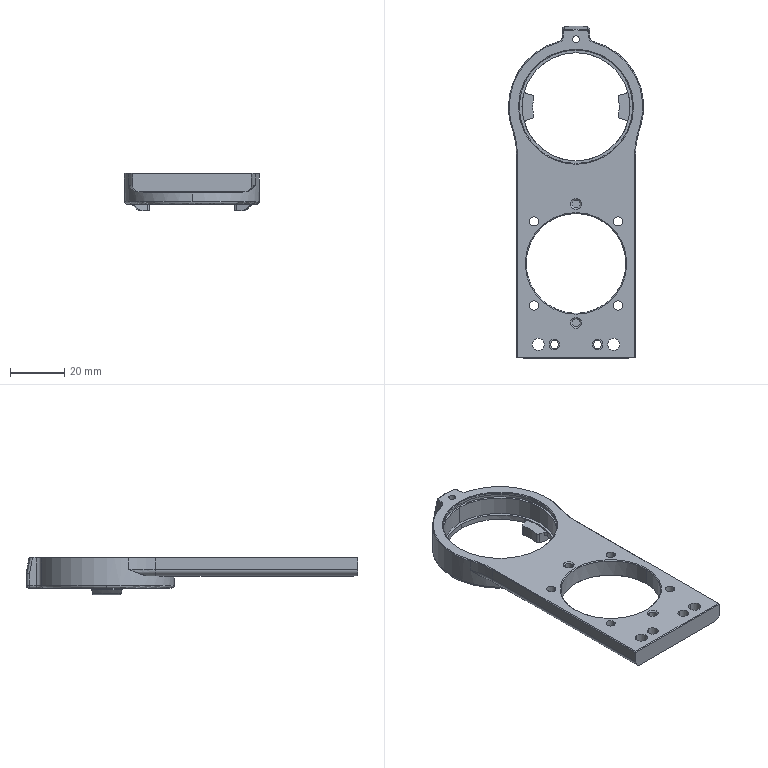NC program | NX | posted with a generic post | part box 50 x 122.9 x 14 mm
Lines 2831 to 4462 of 4462:
(ZLEVEL_PROFILE_COPY , TOOL : D10JING)
N5642 T14 M6
N5644 G54
N5646 G17 G0 G90 X-66.45 Y1.257 S9500 M3
N5648 G43 Z30. H14
N5650 Z-12.5
N5652 G94 G1 Y22.549 Z-13.616 F1000.
N5654 X-66.122 Y23.864 Z-13.687
N5656 X-65.454 Y25.045 Z-13.758
N5658 X-64.495 Y26.004 Z-13.829
N5660 X-63.314 Y26.672 Z-13.9
N5662 X-61.999 Y27. Z-13.971
N5664 X-61.45 Z-14.
N5666 X13.634 F1500.
N5668 G3 X21.777 Y28.364 R25.
N5670 G2 X59.834 Y10. R30.
N5672 G1 X60.172
N5674 G2 X66.114 Y4.83 R6.
N5676 X66.114 Y-4.83 R34.9
N5678 X60.172 Y-10. R6.
N5680 G1 X59.951
N5682 X59.835 Y-9.998
N5684 G2 X21.777 Y-28.364 R30.
N5686 G3 X13.634 Y-27. R25.
N5688 G1 X-61.45
N5690 G2 X-66.45 Y-22. R5.
N5692 G1 Y22.
N5694 G2 X-61.45 Y27. R5.
N5696 G1 Z-12.5
N5698 G0 Z30.
(HOLE_MILLING_COPY_COPY , TOOL : D10JING)
N5700 X31.55 Y0.
N5702 Z0.5
N5704 G41 G1 X27.575 Y-11.323 F1000. D14
N5706 G3 X31.55 Y-16.005 R4.028
N5708 X31.55 Y-16.005 Z-0.5 I0. J16.005 F2000.
N5710 X31.55 Y-16.005 Z-1.5 I0. J16.005
N5712 X31.55 Y-16.005 Z-2.5 I0. J16.005
N5714 X31.55 Y-16.005 Z-3.5 I0. J16.005
N5716 X31.55 Y-16.005 Z-4.5 I0. J16.005
N5718 X31.55 Y-16.005 Z-5.5 I0. J16.005
N5720 X31.55 Y-16.005 Z-6.5 I0. J16.005
N5722 X31.55 Y-16.005 Z-7.5 I0. J16.005
N5724 X31.55 Y-16.005 Z-8.5 I0. J16.005
N5726 X31.55 Y-16.005 Z-9.5 I0. J16.005
N5728 X34.054 Y-15.808 Z-9.525 R16.005
N5730 X47.358 Y2.504 R16.005
N5732 X34.054 Y-15.808 R-16.005
N5734 X37.247 Y-10.561 R4.028
N5736 G40
N5738 G1 X31.55 Y0.
N5740 G0 Z30.
(HOLE_MILLING_COPY_COPY_COPY , TOOL : D10JING)
N5742 Z0.5
N5744 G1 X28.854 Y-12.722 F1000.
N5746 G3 X31.55 Y-16.05 R2.756
N5748 X31.55 Y-16.05 Z-0.5 I0. J16.05 F2000.
N5750 X31.55 Y16.05 Z-1. I0. J16.05
N5752 X15.5 Y0. R16.05
N5754 X31.55 Y16.05 R-16.05
N5756 X28.854 Y12.722 R2.756
N5758 G1 X31.55 Y0.
N5760 G0 Z30.
N5762 M5
(SPOT_DRILLING , TOOL : D6A45)
N5764 T01 M6
N5766 G54
N5768 G17 G0 G90 X-42.006 Y15.556 S9500 M3
N5770 G43 Z30. H1
N5772 G94 G82 G98 Z-1. F250. P200 R3.
N5774 X-56.45 Y14.
N5776 Y8.
N5778 X-48.45 Y0.
N5780 X-56.45 Y-8.
N5782 Y-14.
N5784 X-42.006 Y-15.556
N5786 X-26.45 Y0.
N5788 X-10.894 Y15.556
N5790 X-4.45 Y0.
N5792 X-10.894 Y-15.556
N5794 X31.55 Y0.
N5796 X56.55
N5798 G80
N5800 G0 X56.55 Y0. Z30.
N5802 M5
(DRILLING , TOOL : 4.5ZT)
N5804 T08 M6
N5806 G54
N5808 G17 G0 G90 X-56.45 Y14. S2500 M3
N5810 G43 Z30. H8
N5812 G94 G83 G98 Z-6.452 F200. Q2. R3.
N5814 Y-14.
N5816 G80
N5818 G0 X-56.45 Y-14. Z30.
N5820 M5
(DRILLING_COPY , TOOL : 3.0ZT)
N5822 T16 M6
N5824 G54
N5826 G17 G0 G90 X-56.45 Y8. S2500 M3
N5828 G43 Z30. H16
N5830 G94 G83 G98 Z-9.401 F200. Q2. R3.
N5832 Y-8.
N5834 G80
N5836 G0 X-56.45 Y-8. Z30.
N5838 M5
(DRILLING_COPY_COPY , TOOL : 3.4ZT)
N5840 T07 M6
N5842 G54
N5844 G17 G0 G90 X-42.006 Y15.556 S2500 M3
N5846 G43 Z30. H7
N5848 G94 G83 G98 Z-9.521 F200. Q2. R3.
N5850 Y-15.556
N5852 X-10.894
N5854 Y15.556
N5856 G80
N5858 G0 X-10.894 Y15.556 Z30.
N5860 M5
(DRILLING_COPY_COPY_COPY , TOOL : 2.5ZT)
N5862 T02 M6
N5864 G54
N5866 G17 G0 G90 X56.55 Y0. S2500 M3
N5868 G43 Z30. H2
N5870 G94 G83 G98 Z-13.751 F100. Q2. R3.
N5872 G80
N5874 G0 X56.55 Y0. Z30.
N5876 M5
(HOLE_MILLING_1 , TOOL : D2)
N5878 T17 M6
N5880 G54
N5882 G17 G0 G90 X-56.45 Y8. S9500 M3
N5884 G43 Z30. H17
N5886 Z0.5
N5888 G94 G3 X-56.95 Y7.5 R0.5 F1050.
N5890 X-56.45 Y7. R0.5
N5892 X-56.45 Y7. Z0.35 I0. J1.
N5894 X-56.45 Y7. Z0.2 I0. J1.
N5896 X-56.45 Y7. Z0.05 I0. J1.
N5898 X-56.45 Y7. Z-0.1 I0. J1.
N5900 X-56.45 Y7. Z-0.25 I0. J1.
N5902 X-56.45 Y7. Z-0.4 I0. J1.
N5904 X-56.45 Y7. Z-0.55 I0. J1.
N5906 X-56.45 Y7. Z-0.7 I0. J1.
N5908 X-56.45 Y7. Z-0.85 I0. J1.
N5910 X-56.45 Y7. Z-1. I0. J1.
N5912 X-56.45 Y7. Z-1.15 I0. J1.
N5914 X-56.45 Y7. Z-1.3 I0. J1.
N5916 X-56.45 Y7. Z-1.45 I0. J1.
N5918 X-56.45 Y7. Z-1.6 I0. J1.
N5920 X-56.45 Y7. Z-1.75 I0. J1.
N5922 X-56.45 Y7. Z-1.9 I0. J1.
N5924 X-56.45 Y7. Z-2.05 I0. J1.
N5926 X-56.45 Y7. Z-2.2 I0. J1.
N5928 X-56.45 Y7. Z-2.35 I0. J1.
N5930 X-56.45 Y7. Z-2.5 I0. J1.
N5932 X-56.45 Y7. Z-2.65 I0. J1.
N5934 X-56.45 Y7. Z-2.8 I0. J1.
N5936 X-56.45 Y7. Z-2.95 I0. J1.
N5938 X-56.45 Y7. Z-3.1 I0. J1.
N5940 X-56.45 Y7. Z-3.25 I0. J1.
N5942 X-56.45 Y7. Z-3.4 I0. J1.
N5944 X-56.45 Y7. Z-3.55 I0. J1.
N5946 X-56.45 Y7. Z-3.7 I0. J1.
N5948 X-56.45 Y7. Z-3.85 I0. J1.
N5950 X-56.45 Y7. Z-4. I0. J1.
N5952 X-56.45 Y7. Z-4.15 I0. J1.
N5954 X-56.45 Y7. Z-4.3 I0. J1.
N5956 X-56.45 Y7. Z-4.45 I0. J1.
N5958 X-56.45 Y7. Z-4.6 I0. J1.
N5960 X-56.45 Y7. Z-4.75 I0. J1.
N5962 X-56.45 Y7. Z-4.9 I0. J1.
N5964 X-57.316 Y8.5 Z-5. R-1.
N5966 X-56.95 Y7.134 R1.
N5968 X-57.316 Y8.5 R-1.
N5970 X-57.133 Y7.817 R0.5
N5972 X-56.45 Y8. R0.5
N5974 G0 Z30.
N5976 Y-8.
N5978 Z0.5
N5980 G3 X-56.95 Y-8.5 R0.5
N5982 X-56.45 Y-9. R0.5
N5984 X-56.45 Y-9. Z0.35 I0. J1.
N5986 X-56.45 Y-9. Z0.2 I0. J1.
N5988 X-56.45 Y-9. Z0.05 I0. J1.
N5990 X-56.45 Y-9. Z-0.1 I0. J1.
N5992 X-56.45 Y-9. Z-0.25 I0. J1.
N5994 X-56.45 Y-9. Z-0.4 I0. J1.
N5996 X-56.45 Y-9. Z-0.55 I0. J1.
N5998 X-56.45 Y-9. Z-0.7 I0. J1.
N6000 X-56.45 Y-9. Z-0.85 I0. J1.
N6002 X-56.45 Y-9. Z-1. I0. J1.
N6004 X-56.45 Y-9. Z-1.15 I0. J1.
N6006 X-56.45 Y-9. Z-1.3 I0. J1.
N6008 X-56.45 Y-9. Z-1.45 I0. J1.
N6010 X-56.45 Y-9. Z-1.6 I0. J1.
N6012 X-56.45 Y-9. Z-1.75 I0. J1.
N6014 X-56.45 Y-9. Z-1.9 I0. J1.
N6016 X-56.45 Y-9. Z-2.05 I0. J1.
N6018 X-56.45 Y-9. Z-2.2 I0. J1.
N6020 X-56.45 Y-9. Z-2.35 I0. J1.
N6022 X-56.45 Y-9. Z-2.5 I0. J1.
N6024 X-56.45 Y-9. Z-2.65 I0. J1.
N6026 X-56.45 Y-9. Z-2.8 I0. J1.
N6028 X-56.45 Y-9. Z-2.95 I0. J1.
N6030 X-56.45 Y-9. Z-3.1 I0. J1.
N6032 X-56.45 Y-9. Z-3.25 I0. J1.
N6034 X-56.45 Y-9. Z-3.4 I0. J1.
N6036 X-56.45 Y-9. Z-3.55 I0. J1.
N6038 X-56.45 Y-9. Z-3.7 I0. J1.
N6040 X-56.45 Y-9. Z-3.85 I0. J1.
N6042 X-56.45 Y-9. Z-4. I0. J1.
N6044 X-56.45 Y-9. Z-4.15 I0. J1.
N6046 X-56.45 Y-9. Z-4.3 I0. J1.
N6048 X-56.45 Y-9. Z-4.45 I0. J1.
N6050 X-56.45 Y-9. Z-4.6 I0. J1.
N6052 X-56.45 Y-9. Z-4.75 I0. J1.
N6054 X-56.45 Y-9. Z-4.9 I0. J1.
N6056 X-57.316 Y-7.5 Z-5. R-1.
N6058 X-56.95 Y-8.866 R1.
N6060 X-57.316 Y-7.5 R-1.
N6062 X-57.133 Y-8.183 R0.5
N6064 X-56.45 Y-8. R0.5
N6066 G0 Z30.
N6068 X-48.45 Y0.
N6070 Z0.5
N6072 G3 X-48.705 Y-0.255 R0.255
N6074 X-48.45 Y-0.51 R0.255
N6076 X-48.45 Y-0.51 Z0.35 I0. J0.51
N6078 X-48.45 Y-0.51 Z0.2 I0. J0.51
N6080 X-48.45 Y-0.51 Z0.05 I0. J0.51
N6082 X-48.45 Y-0.51 Z-0.1 I0. J0.51
N6084 X-48.45 Y-0.51 Z-0.25 I0. J0.51
N6086 X-48.45 Y-0.51 Z-0.4 I0. J0.51
N6088 X-48.45 Y-0.51 Z-0.55 I0. J0.51
N6090 X-48.45 Y-0.51 Z-0.7 I0. J0.51
N6092 X-48.45 Y-0.51 Z-0.85 I0. J0.51
N6094 X-48.45 Y-0.51 Z-1. I0. J0.51
N6096 X-48.45 Y-0.51 Z-1.15 I0. J0.51
N6098 X-48.45 Y-0.51 Z-1.3 I0. J0.51
N6100 X-48.45 Y-0.51 Z-1.45 I0. J0.51
N6102 X-48.45 Y-0.51 Z-1.6 I0. J0.51
N6104 X-48.45 Y-0.51 Z-1.75 I0. J0.51
N6106 X-48.45 Y-0.51 Z-1.9 I0. J0.51
N6108 X-48.45 Y-0.51 Z-2.05 I0. J0.51
N6110 X-48.45 Y-0.51 Z-2.2 I0. J0.51
N6112 X-48.45 Y-0.51 Z-2.35 I0. J0.51
N6114 X-48.45 Y-0.51 Z-2.5 I0. J0.51
N6116 X-48.45 Y-0.51 Z-2.65 I0. J0.51
N6118 X-48.45 Y-0.51 Z-2.8 I0. J0.51
N6120 X-48.45 Y-0.51 Z-2.95 I0. J0.51
N6122 X-48.008 Y0.255 Z-3. R0.51
N6124 X-48.705 Y0.442 R0.51
N6126 X-48.008 Y0.255 R-0.51
N6128 X-48.357 Y0.348 R0.255
N6130 X-48.45 Y0. R0.255
N6132 G0 Z30.
N6134 X-4.45
N6136 Z0.5
N6138 G3 X-4.705 Y-0.255 R0.255
N6140 X-4.45 Y-0.51 R0.255
N6142 X-4.45 Y-0.51 Z0.35 I0. J0.51
N6144 X-4.45 Y-0.51 Z0.2 I0. J0.51
N6146 X-4.45 Y-0.51 Z0.05 I0. J0.51
N6148 X-4.45 Y-0.51 Z-0.1 I0. J0.51
N6150 X-4.45 Y-0.51 Z-0.25 I0. J0.51
N6152 X-4.45 Y-0.51 Z-0.4 I0. J0.51
N6154 X-4.45 Y-0.51 Z-0.55 I0. J0.51
N6156 X-4.45 Y-0.51 Z-0.7 I0. J0.51
N6158 X-4.45 Y-0.51 Z-0.85 I0. J0.51
N6160 X-4.45 Y-0.51 Z-1. I0. J0.51
N6162 X-4.45 Y-0.51 Z-1.15 I0. J0.51
N6164 X-4.45 Y-0.51 Z-1.3 I0. J0.51
N6166 X-4.45 Y-0.51 Z-1.45 I0. J0.51
N6168 X-4.45 Y-0.51 Z-1.6 I0. J0.51
N6170 X-4.45 Y-0.51 Z-1.75 I0. J0.51
N6172 X-4.45 Y-0.51 Z-1.9 I0. J0.51
N6174 X-4.45 Y-0.51 Z-2.05 I0. J0.51
N6176 X-4.45 Y-0.51 Z-2.2 I0. J0.51
N6178 X-4.45 Y-0.51 Z-2.35 I0. J0.51
N6180 X-4.45 Y-0.51 Z-2.5 I0. J0.51
N6182 X-4.45 Y-0.51 Z-2.65 I0. J0.51
N6184 X-4.45 Y-0.51 Z-2.8 I0. J0.51
N6186 X-4.45 Y-0.51 Z-2.95 I0. J0.51
N6188 X-4.008 Y0.255 Z-3. R0.51
N6190 X-4.705 Y0.442 R0.51
N6192 X-4.008 Y0.255 R-0.51
N6194 X-4.357 Y0.348 R0.255
N6196 X-4.45 Y0. R0.255
N6198 G0 Z30.
N6200 M5
(ZLEVEL_PROFILE_1 , TOOL : D3R0.5)
N6202 T18 M6
N6204 G54
N6206 G17 G0 G90 X60.519 Y7.649 S9500 M3
N6208 G43 Z30. H18
N6210 Z2.801
N6212 G94 G1 Z-0.199 F1000.
N6214 G3 X60.688 Y5.746 R1.5
N6216 G2 X61.387 Y4.338 R2.517 F2500.
N6218 X61.39 Y-4.327 R30.379
N6220 X60.689 Y-5.746 R2.55
N6222 G1 X60.611 Y-5.826 Z-0.206
N6224 X60.524 Y-5.903 Z-0.212
N6226 X60.432 Y-5.978 Z-0.219
N6228 X60.334 Y-6.05 Z-0.225
N6230 X60.231 Y-6.119 Z-0.232
N6232 X60.123 Y-6.182 Z-0.238
N6234 X60.011 Y-6.241 Z-0.245
N6236 X59.896 Y-6.294 Z-0.251
N6238 X59.779 Y-6.341 Z-0.258
N6240 X59.661 Y-6.382 Z-0.264
N6242 X59.542 Y-6.416 Z-0.271
N6244 X59.424 Y-6.445 Z-0.277
N6246 X59.308 Y-6.467 Z-0.284
N6248 X59.193 Y-6.483 Z-0.291
N6250 X59.081 Y-6.493 Z-0.297
N6252 G3 X61.408 Y-4.334 R2.524
N6254 X61.407 Y4.34 R30.381
N6256 X58.983 Y6.495 R2.515
N6258 G1 X58.862 Y6.499 Z-0.313
N6260 X58.74 Y6.498 Z-0.33
N6262 X58.619 Z-0.346
N6264 X58.498 Z-0.362
N6266 X58.376 Z-0.379
N6268 X58.255 Y6.492 Z-0.395
N6270 X58.377 Y6.498
N6272 X58.965 Y6.493
N6274 G2 X61.426 Y4.343 R2.509
N6276 X61.427 Y-4.342 R30.382
N6278 X58.955 Y-6.495 R2.512
N6280 G1 X58.498 Y-6.498
N6282 Z-0.493
N6284 X58.964 Y-6.496
N6286 G3 X61.448 Y-4.333 R2.522
N6288 X61.446 Y4.344 R30.384
N6290 X58.98 Y6.494 R2.51
N6292 G1 X58.377 Y6.499
N6294 X58.255 Y6.493
N6296 Z-0.591
N6298 X58.377 Y6.499
N6300 X58.996 Y6.495
N6302 G2 X61.465 Y4.344 R2.51
N6304 X61.467 Y-4.333 R30.385
N6306 X58.981 Y-6.496 R2.523
N6308 G1 X58.498 Y-6.498
N6310 Y-6.499 Z-0.689
N6312 X59.002 Y-6.496
N6314 G3 X61.487 Y-4.333 R2.523
N6316 X61.486 Y4.335 R30.388
N6318 X59.002 Y6.496 R2.521
N6320 G1 X58.377 Y6.499
N6322 X58.255 Y6.493
N6324 Y6.499 Z-0.787
N6326 X59.015 Y6.497
N6328 G2 X61.506 Y4.335 R2.522
N6330 X61.507 Y-4.334 R30.391
N6332 X59.023 Y-6.497 R2.522
N6334 G1 X58.498 Y-6.499
N6336 X58.377 Y-6.5 Z-0.885
N6338 X59.043 Y-6.497
N6340 G3 X61.526 Y-4.334 R2.522
N6342 X61.529 Y4.307 R30.401
N6344 X59.104 Y6.497 R2.523
N6346 G1 X58.134 Y6.5
N6348 Z-0.983
N6350 X59.054 Y6.498
N6352 G2 X61.545 Y4.335 R2.523
N6354 X61.546 Y-4.334 R30.401
N6356 X59.062 Y-6.497 R2.522
N6358 G1 X58.377 Y-6.5
N6360 Z-1.082
N6362 X59.082 Y-6.497
N6364 G3 X61.566 Y-4.334 R2.522
N6366 X61.565 Y4.335 R30.408
N6368 X59.074 Y6.498 R2.522
N6370 G1 X58.134 Y6.5
N6372 Z-1.18
N6374 X59.095 Y6.498
N6376 G2 X61.584 Y4.336 R2.522
N6378 X61.585 Y-4.335 R30.414
N6380 X59.102 Y-6.497 R2.521
N6382 G1 X58.377 Y-6.5
N6384 Z-1.278
N6386 X59.121 Y-6.497
N6388 G3 X61.605 Y-4.335 R2.521
N6390 X61.604 Y4.336 R30.42
N6392 X59.114 Y6.498 R2.521
N6394 G1 X58.134 Y6.5
N6396 Z-1.376
N6398 X59.134 Y6.498
N6400 G2 X61.624 Y4.335 R2.522
N6402 X61.625 Y-4.335 R30.426
N6404 X59.14 Y-6.497 R2.521
N6406 G1 X58.377 Y-6.5
N6408 Z-1.474
N6410 X59.159 Y-6.497
N6412 G3 X61.644 Y-4.334 R2.522
N6414 X61.643 Y4.335 R30.432
N6416 X59.153 Y6.498 R2.522
N6418 G1 X58.134 Y6.5
N6420 Z-1.572
N6422 G2 X59.23 Y6.492 R37.923
N6424 X61.663 Y4.339 R2.512
N6426 X61.663 Y-4.342 R30.439
N6428 X59.206 Y-6.492 R2.508
N6430 G1 X58.377 Y-6.5
N6432 Z-1.67
N6434 X59.219 Y-6.493
N6436 G3 X61.683 Y-4.341 R2.51
N6438 X61.682 Y4.337 R30.445
N6440 X59.239 Y6.493 R2.515
N6442 X58.134 Y6.5 R46.951
N6444 G1 Z-1.768
N6446 X59.228 Y6.493
N6448 G2 X61.702 Y4.336 R2.516
N6450 X61.702 Y-4.34 R30.451
N6452 X59.232 Y-6.495 R2.512
N6454 G1 X58.377 Y-6.5
N6456 Z-1.866
N6458 X59.236 Y-6.496
N6460 G3 X61.724 Y-4.329 R2.526
N6462 X61.722 Y4.335 R30.458
N6464 X59.242 Y6.495 R2.518
N6466 G1 X58.134 Y6.5
N6468 Z-1.964
N6470 X59.256 Y6.496
N6472 G2 X61.742 Y4.334 R2.521
N6474 X61.743 Y-4.33 R30.464
N6476 X59.254 Y-6.497 R2.525
N6478 G1 X58.377 Y-6.5
N6480 Z-2.062
N6482 X59.275 Y-6.497
N6484 G3 X61.763 Y-4.332 R2.524
N6486 X61.762 Y4.332 R30.469
N6488 X59.269 Y6.497 R2.524
N6490 G1 X58.134 Y6.5
N6492 Z-2.16
N6494 X59.288 Y6.498
N6496 G2 X61.782 Y4.332 R2.524
N6498 X61.793 Y-4.259 R30.522
N6500 X59.347 Y-6.496 R2.524
N6502 G1 X58.377 Y-6.5
N6504 Z-2.258
N6506 X59.347 Y-6.496
N6508 G3 X61.813 Y-4.259 R2.523
N6510 X61.801 Y4.332 R30.531
N6512 X59.308 Y6.498 R2.524
N6514 G1 X58.134 Y6.5
N6516 Z-2.356
N6518 X59.328 Y6.498
N6520 G2 X61.821 Y4.333 R2.523
N6522 X61.822 Y-4.332 R30.504
N6524 X59.334 Y-6.497 R2.522
N6526 G1 X58.377 Y-6.5
N6528 Z-2.454
N6530 X59.354 Y-6.497
N6532 G3 X61.841 Y-4.333 R2.522
N6534 X61.841 Y4.334 R30.522
N6536 X59.349 Y6.498 R2.522
N6538 G1 X58.134 Y6.5
N6540 Z-2.552
N6542 X59.368 Y6.498
N6544 G2 X61.86 Y4.333 R2.523
N6546 X61.861 Y-4.333 R30.541
N6548 X59.373 Y-6.497 R2.522
N6550 G1 X58.377 Y-6.5
N6552 Z-2.65
N6554 X59.347 Y-6.497
N6556 G3 X61.891 Y-4.259 R2.523
N6558 X61.88 Y4.332 R30.561
N6560 X59.387 Y6.498 R2.523
N6562 G1 X58.134 Y6.5
N6564 Z-2.749
N6566 X59.407 Y6.498
N6568 G2 X61.9 Y4.332 R2.524
N6570 X61.911 Y-4.259 R30.537
N6572 X59.347 Y-6.497 R2.523
N6574 G1 X58.377 Y-6.5
N6576 Z-2.847
N6578 X59.453 Y-6.492
N6580 G3 X61.919 Y-4.339 R2.509
N6582 X61.919 Y4.335 R30.556
N6584 X59.514 Y6.492 R2.515
N6586 G1 X59.347 Y6.498
N6588 X58.134 Y6.5
N6590 Z-2.945
N6592 X59.347 Y6.498
N6594 X59.514 Y6.493
N6596 G2 X61.939 Y4.333 R2.518
N6598 X61.939 Y-4.338 R30.576
N6600 X59.467 Y-6.494 R2.512
N6602 G1 X58.377 Y-6.5
N6604 Z-3.043
N6606 X59.48 Y-6.495
N6608 G3 X61.959 Y-4.338 R2.514
N6610 X61.959 Y4.332 R30.589
N6612 X59.514 Y6.495 R2.52
N6614 G1 X59.347 Y6.498
N6616 X58.134 Y6.5
N6618 Z-3.141
N6620 X59.347 Y6.498
N6622 X59.513 Y6.496
N6624 G2 X61.979 Y4.331 R2.523
N6626 X61.98 Y-4.328 R30.599
N6628 X59.487 Y-6.496 R2.526
N6630 G1 X58.377 Y-6.5
N6632 Z-3.239
N6634 X59.508 Y-6.496
N6636 G3 X61.999 Y-4.329 R2.524
N6638 X61.999 Y4.329 R30.591
N6640 X59.505 Y6.497 R2.525
N6642 G1 X58.134 Y6.5
N6644 Z-3.337
N6646 X59.589 Y6.498
N6648 G2 X62.029 Y4.258 R2.527
N6650 X62.029 Y-4.259 R30.625
N6652 X59.589 Y-6.496 R2.524
N6654 G1 X58.377 Y-6.5
N6656 Z-3.435
N6658 X59.589 Y-6.496
N6660 G3 X62.049 Y-4.259 R2.523
N6662 X62.049 Y4.258 R30.677
N6664 X59.589 Y6.498 R2.526
N6666 G1 X58.134 Y6.5
N6668 Z-3.533
N6670 X59.589 Y6.498
N6672 G2 X62.069 Y4.258 R2.525
N6674 X62.069 Y-4.259 R30.648
N6676 X59.589 Y-6.497 R2.522
N6678 G1 X58.377 Y-6.5
N6680 Z-3.631
N6682 X59.589 Y-6.497
N6684 G3 X62.088 Y-4.259 R2.521
N6686 X62.088 Y4.258 R30.648
N6688 X59.589 Y6.498 R2.524
N6690 G1 X58.134 Y6.5
N6692 Z-3.729
N6694 X59.589 Y6.498
N6696 G2 X62.108 Y4.258 R2.524
N6698 X62.108 Y-4.259 R30.67
N6700 X59.589 Y-6.497 R2.522
N6702 G1 X58.377 Y-6.5
N6704 Z-3.827
N6706 X59.589 Y-6.497
N6708 G3 X62.128 Y-4.259 R2.522
N6710 X62.116 Y4.342 R30.691
N6712 X59.711 Y6.489 R2.503
N6714 G1 X59.347 Y6.5
N6716 X58.134
N6718 Z-3.925
N6720 X59.347
N6722 X59.713 Y6.491
N6724 G2 X62.137 Y4.333 R2.513
N6726 X62.148 Y-4.259 R30.736
N6728 X59.589 Y-6.497 R2.523
N6730 G1 X58.377 Y-6.5
N6732 Z-4.023
N6734 X59.666 Y-6.497
N6736 G3 X62.158 Y-4.329 R2.523
N6738 X62.157 Y4.332 R30.769
N6740 X59.722 Y6.492 R2.514
N6742 G1 X59.347 Y6.5
N6744 X58.134
N6746 Z-4.121
N6748 X59.347
N6750 X59.729 Y6.493
N6752 G2 X62.177 Y4.329 R2.519
N6754 X62.178 Y-4.327 R30.778
N6756 X59.726 Y-6.495 R2.523
N6758 G1 X59.589 Y-6.497
N6760 X58.377 Y-6.5
N6762 Z-4.219
N6764 X59.717 Y-6.495
N6766 G3 X62.197 Y-4.335 R2.514
N6768 X62.197 Y4.328 R30.821
N6770 X59.738 Y6.494 R2.52
N6772 G1 X59.347 Y6.5
N6774 X58.134
N6776 Z-4.317
N6778 X59.347
N6780 X59.747 Y6.496
N6782 G2 X62.217 Y4.328 R2.522
N6784 X62.218 Y-4.325 R30.821
N6786 X59.724 Y-6.496 R2.526
N6788 G1 X58.377 Y-6.5
N6790 Z-4.415
N6792 X59.745 Y-6.496
N6794 G3 X62.237 Y-4.327 R2.524
N6796 X62.237 Y4.327 R30.822
N6798 X59.755 Y6.497 R2.525
N6800 G1 X59.347 Y6.5
N6802 X58.134
N6804 Z-4.514
N6806 X59.347
N6808 G2 X60.074 Y6.477 R4.597
N6810 X62.267 Y4.258 R2.521
N6812 X62.267 Y-4.259 R30.847
N6814 X59.832 Y-6.496 R2.523
N6816 G1 X58.377 Y-6.5
N6818 Z-4.612
N6820 X59.832 Y-6.496
N6822 G3 X62.287 Y-4.259 R2.522
N6824 X62.287 Y4.258 R30.876
N6826 X60.074 Y6.479 R2.519
N6828 X59.347 Y6.5 R5.055
N6830 G1 X58.134
N6832 Z-4.71
N6834 X59.347
N6836 G2 X60.074 Y6.481 R5.615
N6838 X62.307 Y4.258 R2.517
N6840 X62.306 Y-4.259 R30.905
N6842 X59.832 Y-6.497 R2.521
N6844 G1 X58.377 Y-6.5
N6846 Z-4.808
N6848 X59.832 Y-6.497
N6850 G3 X62.326 Y-4.259 R2.52
N6852 X62.326 Y4.258 R30.932
N6854 X60.074 Y6.482 R2.515
N6856 X59.347 Y6.5 R6.317
N6858 G1 X58.134
N6860 Z-4.906
N6862 X59.347
N6864 G2 X60.002 Y6.489 R7.22
N6866 X62.336 Y4.332 R2.514
N6868 X62.346 Y-4.259 R30.959
N6870 X59.832 Y-6.497 R2.52
N6872 G1 X58.377 Y-6.5
N6874 Z-5.004
N6876 X59.832 Y-6.497
N6878 G3 X62.366 Y-4.259 R2.52
N6880 X62.366 Y4.258 R30.987
N6882 X60.074 Y6.486 R2.515
N6884 X59.347 Y6.5 R8.427
N6886 G1 X58.134
N6888 Z-5.102
N6890 X59.589
N6892 X59.958 Y6.491
N6894 G2 X62.375 Y4.338 R2.503
N6896 X62.375 Y-4.338 R31.014
N6898 X59.955 Y-6.491 R2.504
N6900 G1 X59.589 Y-6.5
N6902 X58.377
N6904 Z-5.2
N6906 X59.589
N6908 X59.963 Y-6.493
N6910 G3 X62.395 Y-4.338 R2.505
N6912 X62.395 Y4.338 R31.041
N6914 X59.967 Y6.492 R2.505
N6916 G1 X59.589 Y6.5
N6918 X58.134
N6920 Z-5.298
N6922 X59.589
N6924 X59.966 Y6.494
N6926 G2 X62.416 Y4.326 R2.518
N6928 X62.415 Y-4.337 R31.069
N6930 X59.971 Y-6.494 R2.508
N6932 G1 X59.589 Y-6.5
N6934 X58.377
N6936 Z-5.396
N6938 X59.589
N6940 X59.969 Y-6.496
N6942 G3 X62.436 Y-4.325 R2.521
N6944 X62.436 Y4.326 R31.096
N6946 X59.974 Y6.495 R2.52
N6948 G1 X59.589 Y6.5
N6950 X58.134
N6952 Z-5.494
N6954 X59.589
N6956 G2 X60.317 Y6.467 R4.431
N6958 X62.425 Y4.502 R2.499
N6960 G1 X62.466 Y4.258
N6962 G2 X62.456 Y-4.324 R31.126
N6964 X59.978 Y-6.497 R2.523
N6966 G1 X59.589 Y-6.5
N6968 X58.377
N6970 Z-5.592
N6972 X59.589
N6974 G3 X60.244 Y-6.482 R4.154
N6976 X62.485 Y-4.259 R2.515
N6978 X62.485 Y4.258 R31.157
N6980 G1 X62.444 Y4.502
N6982 G3 X60.317 Y6.469 R2.498
N6984 X59.589 Y6.5 R4.55
N6986 G1 X58.134
N6988 Z-5.69
N6990 X59.589
N6992 G2 X60.394 Y6.462 R3.83
N6994 X62.495 Y4.333 R2.506
N6996 X62.5 Y-4.299 R31.193
N6998 X60.244 Y-6.483 R2.513
N7000 G1 X60.172 Y-6.491
N7002 X59.589 Y-6.5
N7004 X58.377
N7006 Z-5.788
N7008 X59.589
N7010 X60.172 Y-6.493
N7012 X60.244 Y-6.485
N7014 G3 X62.525 Y-4.259 R2.515
N7016 X62.525 Y4.258 R31.167
N7018 G1 X62.5 Y4.424
N7020 G3 X60.317 Y6.475 R2.503
N7022 X59.589 Y6.5 R4.045
N7024 G1 X58.134
N7026 Z-5.886
N7028 X59.589
N7030 G2 X60.346 Y6.474 R4.552
N7032 X62.535 Y4.331 R2.508
N7034 X62.545 Y-4.259 R31.192
N7036 X60.244 Y-6.487 R2.516
N7038 G1 X60.172 Y-6.494
N7040 X59.589 Y-6.5
N7042 X58.377
N7044 Z-5.984
N7046 X59.589
N7048 X60.172 Y-6.496
N7050 X60.244 Y-6.489
N7052 G3 X62.565 Y-4.259 R2.517
N7054 X62.565 Y4.258 R31.218
N7056 X60.317 Y6.48 R2.509
N7058 X59.589 Y6.5 R5.205
N7060 G1 X58.134
N7062 Z-6.082
N7064 X59.589
N7066 G2 X60.317 Y6.482 R6.08
N7068 X62.584 Y4.258 R2.511
N7070 X62.585 Y-4.259 R31.243
N7072 X60.074 Y-6.497 R2.522
N7074 G1 X59.589 Y-6.5
N7076 X58.377
N7078 Z-6.18
N7080 X59.589
N7082 X60.074 Y-6.498
N7084 G3 X62.604 Y-4.259 R2.522
N7086 X62.604 Y4.258 R31.269
N7088 X60.317 Y6.485 R2.514
N7090 X59.589 Y6.5 R7.313
N7092 G1 X58.134
N7094 Z-6.278
N7096 X59.832
N7098 X60.317 Y6.488
N7100 G2 X62.624 Y4.258 R2.516
N7102 X62.624 Y-4.259 R31.294
N7104 X60.172 Y-6.497 R2.521
N7106 G1 X59.832 Y-6.5
N7108 X58.377
N7110 Z-6.376
N7112 X59.832
N7114 X60.172 Y-6.497
N7116 G3 X62.644 Y-4.259 R2.521
N7118 X62.644 Y4.258 R31.319
N7120 X60.317 Y6.49 R2.52
N7122 G1 X59.832 Y6.5
N7124 X58.134
N7126 Z-6.474
N7128 X59.832
N7130 X60.203 Y6.494
N7132 G2 X62.654 Y4.329 R2.513
N7134 X62.664 Y-4.259 R31.362
N7136 X60.172 Y-6.498 R2.521
N7138 G1 X59.832 Y-6.5
N7140 X58.377
N7142 Z-6.573
N7144 X59.832
N7146 X60.172 Y-6.498
N7148 G3 X62.684 Y-4.259 R2.521
N7150 X62.674 Y4.326 R31.388
N7152 X60.205 Y6.496 R2.517
N7154 G1 X59.832 Y6.5
N7156 X58.134
N7158 Z-6.671
N7160 X59.832
N7162 X60.22 Y6.496
N7164 G2 X62.694 Y4.322 R2.522
N7166 X62.704 Y-4.259 R31.414
N7168 X60.172 Y-6.498 R2.521
N7170 G1 X59.832 Y-6.5
N7172 X58.377
N7174 Z-6.753
N7176 X59.832
N7178 X60.172 Y-6.498
N7180 X60.244 Y-6.499
N7182 X60.317 Y-6.496
N7184 G3 X62.72 Y-4.259 R2.519
N7186 X62.711 Y4.324 R31.434
N7188 X60.238 Y6.496 R2.519
N7190 G1 X59.832 Y6.5
N7192 X58.134
N7194 Z-6.835
N7196 X59.832
N7198 X60.317 Y6.496
N7200 G2 X62.736 Y4.258 R2.517
N7202 X62.737 Y-4.259 R31.453
N7204 X60.317 Y-6.496 R2.517
N7206 G1 X60.244 Y-6.499
N7208 X59.832 Y-6.5
N7210 X58.377
N7212 G3 X57.846 Y-6.72 R0.75
N7214 G1 X58.383 Y-8.
N7216 Z-3.835
N7218 G0 Z30.
N7220 X64.184 Y4.801
N7222 Z-3.918
N7224 G1 Z-6.918 F1000.
N7226 G2 X62.349 Y5.364 R1.5
N7228 G3 X60.317 Y6.496 R2.499 F2500.
N7230 G1 X59.832 Y6.5
N7232 X58.134
N7234 Z-7.
N7236 X59.832
N7238 X60.317 Y6.496
N7240 G2 X60.558 Y6.47 R2.5
N7242 G1 X60.761 Y6.448
N7244 X60.797 Y6.421
N7246 X60.812 Y6.417
N7248 X60.833 Y6.432
N7250 X61.066 Y6.367
N7252 X61.105 Y6.355
N7254 X61.442 Y6.207
N7256 G3 X63.24 Y6.675 R1.5
N7258 G1 Z-4.
N7260 G0 Z30.
N7262 X64.19 Y-4.774
N7264 Z-3.918
N7266 G1 Z-6.918 F1000.
N7268 G3 X62.36 Y-5.35 R1.5
N7270 G2 X60.317 Y-6.496 R2.503 F2500.
N7272 G1 X60.244 Y-6.499
N7274 X59.832 Y-6.5
N7276 X58.377
N7278 Z-7.
N7280 X59.832
N7282 X60.244 Y-6.499
N7284 G3 X60.58 Y-6.466 R2.5
N7286 G1 X60.591 Y-6.476
N7288 G3 X60.923 Y-6.406 R1.871
N7290 G1 X61.066 Y-6.367
N7292 X61.106 Y-6.355
N7294 X61.441 Y-6.207
N7296 G2 X63.24 Y-6.677 R1.5
N7298 G1 Z-4.
N7300 G0 Z30.
(ZLEVEL_PROFILE_COPY_1 , TOOL : D3R0.5)
N7302 X57.08 Y8.788
N7304 Z0.
N7306 G1 Z-0.5 F1000.
N7308 X56.735 Y8.406
N7310 G3 X56.672 Y8.113 R0.3
N7312 G2 X57.047 Y6.844 R26.4 F3500.
N7314 G3 X57.627 Y6.4 R0.6
N7316 G1 X58.949
N7318 G3 X59.209 Y6.55 R0.3
N7320 G1 X59.453 Y6.972
N7322 Z0.
N7324 G0 X56.982 Y9.361 Z-0.5
N7326 G1 Z-1. F1000.
N7328 X56.646 Y8.972
N7330 G3 X56.589 Y8.678 R0.3
N7332 G2 X57.144 Y6.87 R26.5 F3500.
N7334 G3 X57.627 Y6.5 R0.5
N7336 G1 X59.041
N7338 G2 X59.448 Y6.467 R2.532
N7340 G3 X59.729 Y6.574 R0.3
N7342 G1 X60.028 Y6.941
N7344 Z-0.5
N7346 G0 X56.978 Y9.373 Z-1.
N7348 G1 Z-1.5 F1000.
N7350 X56.641 Y8.984
N7352 G3 X56.585 Y8.689 R0.3
N7354 G2 X57.144 Y6.87 R26.5 F3500.
N7356 G3 X57.627 Y6.5 R0.5
N7358 G1 X59.143
N7360 G2 X59.497 Y6.475 R2.531
N7362 G3 X59.775 Y6.588 R0.3
N7364 G1 X60.067 Y6.961
N7366 Z-1.
N7368 G0 X56.973 Y9.384 Z-1.5
N7370 G1 Z-2. F1000.
N7372 X56.637 Y8.995
N7374 G3 X56.581 Y8.701 R0.3
N7376 G2 X57.144 Y6.87 R26.5 F3500.
N7378 G3 X57.627 Y6.5 R0.5
N7380 G1 X59.244
N7382 G2 X59.535 Y6.483 R2.53
N7384 G3 X59.81 Y6.603 R0.3
N7386 G1 X60.092 Y6.984
N7388 Z-1.5
N7390 G0 X56.971 Y9.39 Z-2.
N7392 G1 Z-2.5 F1000.
N7394 X56.635 Y9.001
N7396 G3 X56.579 Y8.707 R0.3
N7398 G2 X57.144 Y6.87 R26.5 F3500.
N7400 G3 X57.627 Y6.5 R0.5
N7402 G1 X59.343
N7404 G2 X59.574 Y6.489 R2.539
N7406 G3 X59.846 Y6.614 R0.3
N7408 G1 X60.12 Y7.001
N7410 Z-2.
N7412 G0 X56.969 Y9.396 Z-2.5
N7414 G1 Z-3. F1000.
N7416 X56.633 Y9.007
N7418 G3 X56.577 Y8.713 R0.3
N7420 G2 X57.144 Y6.87 R26.5 F3500.
N7422 G3 X57.627 Y6.5 R0.5
N7424 G1 X59.444
N7426 X59.603 Y6.495
N7428 G3 X59.872 Y6.628 R0.3
N7430 G1 X60.134 Y7.022
N7432 Z-2.5
N7434 G0 X56.967 Y9.402 Z-3.
N7436 G1 Z-3.5 F1000.
N7438 X56.631 Y9.013
N7440 G3 X56.575 Y8.719 R0.3
N7442 G2 X57.144 Y6.87 R26.5 F3500.
N7444 G3 X57.627 Y6.5 R0.5
N7446 G1 X59.547
N7448 X59.633 Y6.498
N7450 G3 X59.898 Y6.639 R0.3
N7452 G1 X60.149 Y7.041
N7454 Z-3.
N7456 G0 X56.965 Y9.407 Z-3.5
N7458 G1 Z-4. F1000.
N7460 X56.629 Y9.018
N7462 G3 X56.573 Y8.723 R0.3
N7464 G2 X57.144 Y6.87 R26.5 F3500.
N7466 G3 X57.627 Y6.5 R0.5
N7468 G1 X59.657
N7470 G3 X59.917 Y6.649 R0.3
N7472 G1 X60.155 Y7.059
N7474 Z-3.5
N7476 G0 X56.965 Y9.407 Z-4.
N7478 G1 Z-4.5 F1000.
N7480 X56.629 Y9.018
N7482 G3 X56.573 Y8.723 R0.3
N7484 G2 X57.144 Y6.87 R26.5 F3500.
N7486 G3 X57.627 Y6.5 R0.5
N7488 G1 X59.658
N7490 G3 X59.918 Y6.65 R0.3
N7492 G1 X60.161 Y7.071
N7494 Z-4.
N7496 G0 X56.963 Y9.412 Z-4.5
N7498 G1 Z-5. F1000.
N7500 X56.628 Y9.023
N7502 G3 X56.571 Y8.728 R0.3
N7504 G2 X57.144 Y6.87 R26.5 F3500.
N7506 G3 X57.627 Y6.5 R0.5
N7508 G1 X59.683
N7510 G3 X59.943 Y6.65 R0.3
N7512 G1 X60.191 Y7.079
N7514 Z-4.5
N7516 G0 X56.963 Y9.412 Z-4.953
N7518 G1 Z-5.453 F1000.
N7520 X56.628 Y9.023
N7522 G3 X56.571 Y8.728 R0.3
N7524 G2 X57.144 Y6.87 R26.5 F3500.
N7526 G3 X57.627 Y6.5 R0.5
N7528 G1 X59.683
N7530 G3 X59.943 Y6.65 R0.3
N7532 G1 X60.196 Y7.088
N7534 Z-4.953
N7536 G0 X56.963 Y9.412 Z-5.405
N7538 G1 Z-5.905 F1000.
N7540 X56.628 Y9.023
N7542 G3 X56.571 Y8.728 R0.3
N7544 G2 X57.144 Y6.87 R26.5 F3500.
N7546 G3 X57.627 Y6.5 R0.5
N7548 G1 X59.683
N7550 G3 X59.943 Y6.65 R0.3
N7552 G1 X60.2 Y7.096
N7554 Z-5.405
N7556 G0 X56.963 Y9.412 Z-5.858
N7558 G1 Z-6.358 F1000.
N7560 X56.628 Y9.023
N7562 G3 X56.571 Y8.728 R0.3
N7564 G2 X57.144 Y6.87 R26.5 F3500.
N7566 G3 X57.627 Y6.5 R0.5
N7568 G1 X59.683
N7570 G3 X59.943 Y6.65 R0.3
N7572 G1 X60.203 Y7.099
N7574 Z-5.858
N7576 G0 X56.963 Y9.412 Z-6.31
N7578 G1 Z-6.81 F1000.
N7580 X56.628 Y9.023
N7582 G3 X56.571 Y8.728 R0.3
N7584 G2 X57.144 Y6.87 R26.5 F3500.
N7586 G3 X57.627 Y6.5 R0.5
N7588 G1 X59.683
N7590 G3 X59.943 Y6.65 R0.3
N7592 G1 X60.203 Y7.1
N7594 Z-6.31
N7596 G0 X56.963 Y9.412 Z-6.763
N7598 G1 Z-7.263 F1000.
N7600 X56.628 Y9.023
N7602 G3 X56.571 Y8.728 R0.3
N7604 G2 X57.144 Y6.87 R26.5 F3500.
N7606 G3 X57.627 Y6.5 R0.5
N7608 G1 X59.683
N7610 G3 X59.943 Y6.65 R0.3
N7612 G1 X60.203 Y7.1
N7614 Z-6.763
N7616 G0 X56.963 Y9.412 Z-7.215
N7618 G1 Z-7.715 F1000.
N7620 X56.628 Y9.023
N7622 G3 X56.571 Y8.728 R0.3
N7624 G2 X57.144 Y6.87 R26.5 F3500.
N7626 G3 X57.627 Y6.5 R0.5
N7628 G1 X59.683
N7630 G3 X59.943 Y6.65 R0.3
N7632 G1 X60.203 Y7.1
N7634 Z-7.215
N7636 G0 X56.963 Y9.412 Z-7.668
N7638 G1 Z-8.168 F1000.
N7640 X56.628 Y9.023
N7642 G3 X56.571 Y8.728 R0.3
N7644 G2 X57.144 Y6.87 R26.5 F3500.
N7646 G3 X57.627 Y6.5 R0.5
N7648 G1 X59.683
N7650 G3 X59.943 Y6.65 R0.3
N7652 G1 X60.203 Y7.1
N7654 Z-7.668
N7656 G0 X56.963 Y9.412 Z-8.12
N7658 G1 Z-8.62 F1000.
N7660 X56.628 Y9.023
N7662 G3 X56.571 Y8.728 R0.3
N7664 G2 X57.144 Y6.87 R26.5 F3500.
N7666 G3 X57.627 Y6.5 R0.5
N7668 G1 X59.683
N7670 G3 X59.943 Y6.65 R0.3
N7672 G1 X60.203 Y7.1
N7674 Z-8.12
N7676 G0 X56.963 Y9.412 Z-8.573
N7678 G1 Z-9.073 F1000.
N7680 X56.628 Y9.023
N7682 G3 X56.571 Y8.728 R0.3
N7684 G2 X57.144 Y6.87 R26.5 F3500.
N7686 G3 X57.627 Y6.5 R0.5
N7688 G1 X59.683
N7690 G3 X59.943 Y6.65 R0.3
N7692 G1 X60.203 Y7.1
N7694 Z-8.573
N7696 G0 X56.963 Y9.412 Z-9.025
N7698 G1 Z-9.525 F1000.
N7700 X56.628 Y9.023
N7702 G3 X56.571 Y8.728 R0.3
N7704 G2 X57.144 Y6.87 R26.5 F3500.
N7706 G3 X57.627 Y6.5 R0.5
N7708 G1 X59.683
N7710 G3 X59.943 Y6.65 R0.3
N7712 G1 X60.203 Y7.1
N7714 Z-9.025
N7716 G0 X56.963 Y9.412 Z-9.5
N7718 G1 Z-10. F1000.
N7720 X56.628 Y9.023
N7722 G3 X56.571 Y8.728 R0.3
N7724 G2 X57.144 Y6.87 R26.5 F3500.
N7726 G3 X57.627 Y6.5 R0.5
N7728 G1 X59.683
N7730 G3 X59.943 Y6.65 R0.3
N7732 G1 X60.203 Y7.1
N7734 Z-9.5
N7736 G0 X56.963 Y9.412 Z-10.
N7738 G1 Z-10.5 F1000.
N7740 X56.628 Y9.023
N7742 G3 X56.571 Y8.728 R0.3
N7744 G2 X57.144 Y6.87 R26.5 F3500.
N7746 G3 X57.627 Y6.5 R0.5
N7748 G1 X59.683
N7750 G3 X59.943 Y6.65 R0.3
N7752 G1 X60.203 Y7.1
N7754 Z-10.
N7756 G0 X56.963 Y9.412 Z-10.5
N7758 G1 Z-11. F1000.
N7760 X56.628 Y9.023
N7762 G3 X56.571 Y8.728 R0.3
N7764 G2 X57.144 Y6.87 R26.5 F3500.
N7766 G3 X57.627 Y6.5 R0.5
N7768 G1 X59.683
N7770 G3 X59.943 Y6.65 R0.3
N7772 G1 X60.203 Y7.1
N7774 Z-10.5
N7776 G0 X56.956 Y9.431 Z-11.
N7778 G1 Z-11.5 F1000.
N7780 X56.621 Y9.042
N7782 G3 X56.565 Y8.747 R0.3
N7784 G2 X57.144 Y6.87 R26.5 F3500.
N7786 G3 X57.627 Y6.5 R0.5
N7788 G1 X59.686
N7790 G3 X59.946 Y6.65 R0.3
N7792 G1 X60.205 Y7.1
N7794 Z-11.
N7796 G0 Z30.
N7798 X59.457 Y-6.972
N7800 Z0.
N7802 G1 Z-0.5 F1000.
N7804 X59.213 Y-6.55
N7806 G3 X58.953 Y-6.4 R0.3
N7808 G1 X57.627 F3500.
N7810 G3 X57.047 Y-6.844 R0.6
N7812 G2 X56.672 Y-8.115 R26.4
N7814 G3 X56.735 Y-8.408 R0.3
N7816 G1 X57.079 Y-8.789
N7818 Z0.
N7820 G0 X60.037 Y-6.937 Z-0.5
N7822 G1 Z-1. F1000.
N7824 X59.736 Y-6.571
N7826 G3 X59.455 Y-6.466 R0.3
N7828 G2 X59.041 Y-6.5 R2.534 F3500.
N7830 G1 X57.627
N7832 G3 X57.144 Y-6.87 R0.5
N7834 G2 X56.588 Y-8.679 R26.5
N7836 G3 X56.645 Y-8.974 R0.3
N7838 G1 X56.981 Y-9.362
N7840 Z-0.5
N7842 G0 X60.06 Y-6.963 Z-1.
N7844 G1 Z-1.5 F1000.
N7846 X59.769 Y-6.589
N7848 G3 X59.491 Y-6.476 R0.3
N7850 G2 X59.143 Y-6.5 R2.53 F3500.
N7852 G1 X57.627
N7854 G3 X57.144 Y-6.87 R0.5
N7856 G2 X56.585 Y-8.688 R26.5
N7858 G3 X56.642 Y-8.983 R0.3
N7860 G1 X56.978 Y-9.371
N7862 Z-1.
N7864 G0 X60.079 Y-6.987 Z-1.5
N7866 G1 Z-2. F1000.
N7868 X59.799 Y-6.605
N7870 G3 X59.524 Y-6.485 R0.3
N7872 G2 X59.244 Y-6.5 R2.529 F3500.
N7874 G1 X57.627
N7876 G3 X57.144 Y-6.87 R0.5
N7878 G2 X56.583 Y-8.696 R26.5
N7880 G3 X56.639 Y-8.99 R0.3
N7882 G1 X56.975 Y-9.379
N7884 Z-1.5
N7886 G0 X60.1 Y-7.006 Z-2.
N7888 G1 Z-2.5 F1000.
N7890 X59.829 Y-6.618
N7892 G3 X59.557 Y-6.491 R0.3
N7894 G2 X59.343 Y-6.5 R2.538 F3500.
N7896 G1 X57.627
N7898 G3 X57.144 Y-6.87 R0.5
N7900 G2 X56.58 Y-8.703 R26.5
N7902 G3 X56.636 Y-8.998 R0.3
N7904 G1 X56.972 Y-9.387
N7906 Z-2.
N7908 G0 X60.12 Y-7.026 Z-2.5
N7910 G1 Z-3. F1000.
N7912 X59.859 Y-6.63
N7914 G3 X59.591 Y-6.496 R0.3
N7916 G1 X59.444 Y-6.5 F3500.
N7918 X57.627
N7920 G3 X57.144 Y-6.87 R0.5
N7922 G2 X56.578 Y-8.71 R26.5
N7924 G3 X56.634 Y-9.005 R0.3
N7926 G1 X56.97 Y-9.394
N7928 Z-2.5
N7930 G0 X60.141 Y-7.043 Z-3.
N7932 G1 Z-3.5 F1000.
N7934 X59.891 Y-6.64
N7936 G3 X59.626 Y-6.499 R0.3
N7938 G1 X59.547 Y-6.5 F3500.
N7940 X57.627
N7942 G3 X57.144 Y-6.87 R0.5
N7944 G2 X56.575 Y-8.717 R26.5
N7946 G3 X56.631 Y-9.012 R0.3
N7948 G1 X56.967 Y-9.401
N7950 Z-3.
N7952 G0 X60.155 Y-7.059 Z-3.5
N7954 G1 Z-4. F1000.
N7956 X59.917 Y-6.649
N7958 G3 X59.657 Y-6.5 R0.3
N7960 G1 X57.627 F3500.
N7962 G3 X57.144 Y-6.87 R0.5
N7964 G2 X56.573 Y-8.723 R26.5
N7966 G3 X56.629 Y-9.018 R0.3
N7968 G1 X56.965 Y-9.407
N7970 Z-3.5
N7972 G0 X60.16 Y-7.072 Z-4.
N7974 G1 Z-4.5 F1000.
N7976 X59.917 Y-6.65
N7978 G3 X59.657 Y-6.5 R0.3
N7980 G1 X57.627 F3500.
N7982 G3 X57.144 Y-6.87 R0.5
N7984 G2 X56.573 Y-8.723 R26.5
N7986 G3 X56.629 Y-9.018 R0.3
N7988 G1 X56.965 Y-9.407
N7990 Z-4.
N7992 G0 X60.166 Y-7.082 Z-4.5
N7994 G1 Z-5. F1000.
N7996 X59.917 Y-6.65
N7998 G3 X59.657 Y-6.5 R0.3
N8000 G1 X57.627 F3500.
N8002 G3 X57.144 Y-6.87 R0.5
N8004 G2 X56.573 Y-8.723 R26.5
N8006 G3 X56.629 Y-9.018 R0.3
N8008 G1 X56.965 Y-9.407
N8010 Z-4.5
N8012 G0 X60.172 Y-7.091 Z-4.953
N8014 G1 Z-5.453 F1000.
N8016 X59.917 Y-6.65
N8018 G3 X59.657 Y-6.5 R0.3
N8020 G1 X57.627 F3500.
N8022 G3 X57.144 Y-6.87 R0.5
N8024 G2 X56.573 Y-8.723 R26.5
N8026 G3 X56.629 Y-9.018 R0.3
N8028 G1 X56.965 Y-9.407
N8030 Z-4.953
N8032 G0 X60.176 Y-7.097 Z-5.405
N8034 G1 Z-5.905 F1000.
N8036 X59.917 Y-6.65
N8038 G3 X59.658 Y-6.5 R0.3
N8040 G1 X57.627 F3500.
N8042 G3 X57.144 Y-6.87 R0.5
N8044 G2 X56.573 Y-8.723 R26.5
N8046 G3 X56.629 Y-9.018 R0.3
N8048 G1 X56.965 Y-9.407
N8050 Z-5.405
N8052 G0 X60.177 Y-7.1 Z-5.858
N8054 G1 Z-6.358 F1000.
N8056 X59.918 Y-6.65
N8058 G3 X59.658 Y-6.5 R0.3
N8060 G1 X57.627 F3500.
N8062 G3 X57.144 Y-6.87 R0.5
N8064 G2 X56.573 Y-8.723 R26.5
N8066 G3 X56.629 Y-9.018 R0.3
N8068 G1 X56.965 Y-9.407
N8070 Z-5.858
N8072 G0 X60.178 Y-7.1 Z-6.31
N8074 G1 Z-6.81 F1000.
N8076 X59.918 Y-6.65
N8078 G3 X59.658 Y-6.5 R0.3
N8080 G1 X57.627 F3500.
N8082 G3 X57.144 Y-6.87 R0.5
N8084 G2 X56.573 Y-8.723 R26.5
N8086 G3 X56.629 Y-9.018 R0.3
N8088 G1 X56.965 Y-9.407
N8090 Z-6.31
N8092 G0 X60.178 Y-7.1 Z-6.763
N8094 G1 Z-7.263 F1000.
N8096 X59.918 Y-6.65
N8098 G3 X59.658 Y-6.5 R0.3
N8100 G1 X57.627 F3500.
N8102 G3 X57.144 Y-6.87 R0.5
N8104 G2 X56.573 Y-8.723 R26.5
N8106 G3 X56.629 Y-9.018 R0.3
N8108 G1 X56.965 Y-9.407
N8110 Z-6.763
N8112 G0 X60.178 Y-7.1 Z-7.215
N8114 G1 Z-7.715 F1000.
N8116 X59.918 Y-6.65
N8118 G3 X59.658 Y-6.5 R0.3
N8120 G1 X57.627 F3500.
N8122 G3 X57.144 Y-6.87 R0.5
N8124 G2 X56.573 Y-8.723 R26.5
N8126 G3 X56.629 Y-9.018 R0.3
N8128 G1 X56.965 Y-9.407
N8130 Z-7.215
N8132 G0 X60.178 Y-7.1 Z-7.668
N8134 G1 Z-8.168 F1000.
N8136 X59.918 Y-6.65
N8138 G3 X59.659 Y-6.5 R0.3
N8140 G1 X57.627 F3500.
N8142 G3 X57.144 Y-6.87 R0.5
N8144 G2 X56.573 Y-8.723 R26.5
N8146 G3 X56.629 Y-9.018 R0.3
N8148 G1 X56.965 Y-9.407
N8150 Z-7.668
N8152 G0 X60.178 Y-7.1 Z-8.12
N8154 G1 Z-8.62 F1000.
N8156 X59.919 Y-6.65
N8158 G3 X59.659 Y-6.5 R0.3
N8160 G1 X57.627 F3500.
N8162 G3 X57.144 Y-6.87 R0.5
N8164 G2 X56.573 Y-8.723 R26.5
N8166 G3 X56.629 Y-9.018 R0.3
N8168 G1 X56.965 Y-9.407
N8170 Z-8.12
N8172 G0 X60.179 Y-7.1 Z-8.573
N8174 G1 Z-9.073 F1000.
N8176 X59.919 Y-6.65
N8178 G3 X59.659 Y-6.5 R0.3
N8180 G1 X57.627 F3500.
N8182 G3 X57.144 Y-6.87 R0.5
N8184 G2 X56.573 Y-8.724 R26.5
N8186 G3 X56.629 Y-9.018 R0.3
N8188 G1 X56.965 Y-9.407
N8190 Z-8.573
N8192 G0 X60.179 Y-7.1 Z-9.025
N8194 G1 Z-9.525 F1000.
N8196 X59.919 Y-6.65
N8198 G3 X59.659 Y-6.5 R0.3
N8200 G1 X57.627 F3500.
N8202 G3 X57.144 Y-6.87 R0.5
N8204 G2 X56.573 Y-8.724 R26.5
N8206 G3 X56.629 Y-9.018 R0.3
N8208 G1 X56.965 Y-9.407
N8210 Z-9.025
N8212 G0 X60.179 Y-7.1 Z-9.5
N8214 G1 Z-10. F1000.
N8216 X59.919 Y-6.65
N8218 G3 X59.659 Y-6.5 R0.3
N8220 G1 X57.627 F3500.
N8222 G3 X57.144 Y-6.87 R0.5
N8224 G2 X56.573 Y-8.724 R26.5
N8226 G3 X56.629 Y-9.018 R0.3
N8228 G1 X56.965 Y-9.407
N8230 Z-9.5
N8232 G0 X60.179 Y-7.1 Z-10.
N8234 G1 Z-10.5 F1000.
N8236 X59.919 Y-6.65
N8238 G3 X59.66 Y-6.5 R0.3
N8240 G1 X57.627 F3500.
N8242 G3 X57.144 Y-6.87 R0.5
N8244 G2 X56.573 Y-8.724 R26.5
N8246 G3 X56.629 Y-9.018 R0.3
N8248 G1 X56.965 Y-9.408
N8250 Z-10.
N8252 G0 X60.179 Y-7.1 Z-10.5
N8254 G1 Z-11. F1000.
N8256 X59.92 Y-6.65
N8258 G3 X59.66 Y-6.5 R0.3
N8260 G1 X57.627 F3500.
N8262 G3 X57.144 Y-6.87 R0.5
N8264 G2 X56.573 Y-8.724 R26.5
N8266 G3 X56.629 Y-9.018 R0.3
N8268 G1 X56.965 Y-9.408
N8270 Z-10.5
N8272 G0 X60.186 Y-7.1 Z-11.
N8274 G1 Z-11.5 F1000.
N8276 X59.926 Y-6.65
N8278 G3 X59.667 Y-6.5 R0.3
N8280 G1 X57.627 F3500.
N8282 G3 X57.144 Y-6.87 R0.5
N8284 G2 X56.569 Y-8.736 R26.5
N8286 G3 X56.625 Y-9.031 R0.3
N8288 G1 X56.96 Y-9.42
N8290 Z-11.
N8292 G0 Z30.
N8294 M5
(PLANAR_PROFILE , TOOL : D6A45)
N8296 T01 M6
N8298 G54
N8300 G17 G0 G90 X56.595 Y0.3 S9500 M3
N8302 G43 Z30. H1
N8304 Z0.5
N8306 G94 G1 X56.413 Z0.451 F1500.
N8308 X56.25 Y0.137 Z0.389
N8310 Y-0.137 Z0.316
N8312 X56.413 Y-0.3 Z0.254
N8314 X56.687 Z0.181
N8316 X56.85 Y-0.137 Z0.119
N8318 Y0.137 Z0.045
N8320 X56.687 Y0.3 Z-0.016
N8322 X56.413 Z-0.09
N8324 X56.25 Y0.137 Z-0.152
N8326 Y-0.137 Z-0.225
N8328 X56.413 Y-0.3 Z-0.287
N8330 X56.687 Z-0.361
N8332 X56.85 Y-0.137 Z-0.422
N8334 Y0.137 Z-0.496
N8336 X56.687 Y0.3 Z-0.557
N8338 X56.413 Z-0.631
N8340 X56.25 Y0.137 Z-0.693
N8342 Y-0.137 Z-0.766
N8344 X56.413 Y-0.3 Z-0.828
N8346 X56.687 Z-0.902
N8348 X56.85 Y-0.137 Z-0.963
N8350 Y0. Z-1.
N8352 G3 X56.55 Y0.3 R0.3
N8354 X56.85 Y0. R-0.3
N8356 X56.7 Y0.26 R0.3
N8358 G1 Z0.5
N8360 G0 Z30.
N8362 X50.877 Y-0.937
N8364 Z0.5
N8366 G1 Z-1.
N8368 X51.6 Y-0.52
N8370 G3 X51.9 Y0. R0.6
N8372 X31.55 Y20.35 R20.35
N8374 X51.9 Y0. R-20.35
N8376 X51.6 Y0.52 R0.6
N8378 G1 X50.877 Y0.937
N8380 Z0.5
N8382 G0 Z30.
N8384 X61.94 Y0.916
N8386 Z0.5
N8388 G1 Z-1.
N8390 X61.254 Y0.52
N8392 G3 X60.954 Y0. R0.6
N8394 G2 X60.878 Y-2.123 R29.491
N8396 X60.649 Y-4.234 R29.63
N8398 X60.08 Y-5.257 R1.643
N8400 X59.002 Y-5.65 R1.675
N8402 G1 X57.627
N8404 G3 X56.323 Y-6.65 R1.35
N8406 G2 X23.194 Y-24.251 R25.65
N8408 G3 X13.634 Y-22.65 R29.35
N8410 G1 X-61.1
N8412 G2 X-62.1 Y-21.65 R1.
N8414 G1 Y21.65
N8416 G2 X-61.1 Y22.65 R1.
N8418 G1 X13.634
N8420 G3 X23.194 Y24.251 R29.35
N8422 G2 X56.323 Y6.65 R25.65
N8424 G3 X57.627 Y5.65 R1.35
N8426 G1 X59.002
N8428 G2 X60.08 Y5.257 R1.675
N8430 X60.649 Y4.234 R1.644
N8432 X60.878 Y2.123 R29.63
N8434 X60.954 Y0. R29.491
N8436 G3 X61.254 Y-0.52 R0.6
N8438 G1 X61.94 Y-0.916
N8440 Z0.5
N8442 G0 Z30.
N8444 X-10.267 Y15.981
N8446 Z0.5
N8448 G1 X-10.342 Y16.108 Z0.46
N8450 X-10.679 Y16.306 Z0.356
N8452 X-11.108 Z0.241
N8454 X-11.445 Y16.108 Z0.136
N8456 X-11.644 Y15.771 Z0.031
N8458 Y15.342 Z-0.084
N8460 X-11.445 Y15.005 Z-0.189
N8462 X-11.108 Y14.806 Z-0.294
N8464 X-10.679 Z-0.408
N8466 X-10.342 Y15.005 Z-0.513
N8468 X-10.144 Y15.342 Z-0.618
N8470 Y15.771 Z-0.733
N8472 X-10.342 Y16.108 Z-0.838
N8474 X-10.679 Y16.306 Z-0.943
N8476 X-10.894 Z-1.
N8478 G3 X-11.644 Y15.556 R0.75
N8480 X-10.894 Y16.306 R-0.75
N8482 X-11.413 Y16.006 R0.6
N8484 G1 Z0.5
N8486 G0 Z30.
N8488 X-4.409 Y-0.028
N8490 Z0.5
N8492 G1 Z-1.
N8494 X-3.7 Y-0.52
N8496 G3 X-3.4 Y0. R0.6
N8498 X-4.45 Y1.05 R1.05
N8500 X-3.4 Y0. R-1.05
N8502 X-3.7 Y0.52 R0.6
N8504 G1 X-4.409 Y0.028
N8506 Z0.5
N8508 G0 Z30.
N8510 X-11.52 Y-15.981
N8512 Z0.5
N8514 G1 X-11.445 Y-16.108 Z0.46
N8516 X-11.108 Y-16.306 Z0.356
N8518 X-10.679 Z0.241
N8520 X-10.342 Y-16.108 Z0.136
N8522 X-10.144 Y-15.771 Z0.031
N8524 Y-15.342 Z-0.084
N8526 X-10.342 Y-15.005 Z-0.189
N8528 X-10.679 Y-14.806 Z-0.294
N8530 X-11.108 Z-0.408
N8532 X-11.445 Y-15.005 Z-0.513
N8534 X-11.644 Y-15.342 Z-0.618
N8536 Y-15.771 Z-0.733
N8538 X-11.445 Y-16.108 Z-0.838
N8540 X-11.108 Y-16.306 Z-0.943
N8542 X-10.894 Z-1.
N8544 G3 X-10.144 Y-15.556 R0.75
N8546 X-10.894 Y-16.306 R-0.75
N8548 X-10.374 Y-16.006 R0.6
N8550 G1 Z0.5
N8552 G0 Z30.
N8554 X-9.626 Y-0.939
N8556 Z0.5
N8558 G1 Z-1.
N8560 X-8.9 Y-0.52
N8562 G3 X-8.6 Y0. R0.6
N8564 X-26.45 Y17.85 R17.85
N8566 X-8.6 Y0. R-17.85
N8568 X-8.9 Y0.52 R0.6
N8570 G1 X-9.626 Y0.939
N8572 Z0.5
N8574 G0 Z30.
N8576 X-42.633 Y-15.981
N8578 Z0.5
N8580 G1 X-42.558 Y-16.108 Z0.46
N8582 X-42.221 Y-16.306 Z0.356
N8584 X-41.792 Z0.241
N8586 X-41.455 Y-16.108 Z0.136
N8588 X-41.256 Y-15.771 Z0.031
N8590 Y-15.342 Z-0.084
N8592 X-41.455 Y-15.005 Z-0.189
N8594 X-41.792 Y-14.806 Z-0.294
N8596 X-42.221 Z-0.408
N8598 X-42.558 Y-15.005 Z-0.513
N8600 X-42.756 Y-15.342 Z-0.618
N8602 Y-15.771 Z-0.733
N8604 X-42.558 Y-16.108 Z-0.838
N8606 X-42.221 Y-16.306 Z-0.943
N8608 X-42.006 Z-1.
N8610 G3 X-41.256 Y-15.556 R0.75
N8612 X-42.006 Y-16.306 R-0.75
N8614 X-41.487 Y-16.006 R0.6
N8616 G1 Z0.5
N8618 G0 Z30.
N8620 X-56.716 Y-13.862
N8622 Z0.5
N8624 G1 Z-1.
N8626 X-57.45 Y-13.48
N8628 G3 X-57.75 Y-14. R0.6
N8630 X-56.45 Y-15.3 R1.3
N8632 X-57.75 Y-14. R-1.3
N8634 X-57.45 Y-14.52 R0.6
N8636 G1 X-56.716 Y-14.138
N8638 Z0.5
N8640 G0 Z30.
N8642 X-56.409 Y-8.028
N8644 Z0.5
N8646 G1 Z-1.
N8648 X-55.7 Y-8.52
N8650 G3 X-55.4 Y-8. R0.6
N8652 X-56.45 Y-6.95 R1.05
N8654 X-55.4 Y-8. R-1.05
N8656 X-55.7 Y-7.48 R0.6
N8658 G1 X-56.409 Y-7.972
N8660 Z0.5
N8662 G0 Z30.
N8664 X-48.409 Y-0.028
N8666 Z0.5
N8668 G1 Z-1.
N8670 X-47.7 Y-0.52
N8672 G3 X-47.4 Y0. R0.6
N8674 X-48.45 Y1.05 R1.05
N8676 X-47.4 Y0. R-1.05
N8678 X-47.7 Y0.52 R0.6
N8680 G1 X-48.409 Y0.028
N8682 Z0.5
N8684 G0 Z30.
N8686 X-56.409 Y7.972
N8688 Z0.5
N8690 G1 Z-1.
N8692 X-55.7 Y7.48
N8694 G3 X-55.4 Y8. R0.6
N8696 X-56.45 Y9.05 R1.05
N8698 X-55.4 Y8. R-1.05
N8700 X-55.7 Y8.52 R0.6
N8702 G1 X-56.409 Y8.028
N8704 Z0.5
N8706 G0 Z30.
N8708 X-56.716 Y14.138
N8710 Z0.5
N8712 G1 Z-1.
N8714 X-57.45 Y14.52
N8716 G3 X-57.75 Y14. R0.6
N8718 X-56.45 Y12.7 R1.3
N8720 X-57.75 Y14. R-1.3
N8722 X-57.45 Y13.48 R0.6
N8724 G1 X-56.716 Y13.862
N8726 Z0.5
N8728 G0 Z30.
N8730 X-41.38 Y15.981
N8732 Z0.5
N8734 G1 X-41.455 Y16.108 Z0.46
N8736 X-41.792 Y16.306 Z0.356
N8738 X-42.221 Z0.241
N8740 X-42.558 Y16.108 Z0.136
N8742 X-42.756 Y15.771 Z0.031
N8744 Y15.342 Z-0.084
N8746 X-42.558 Y15.005 Z-0.189
N8748 X-42.221 Y14.806 Z-0.294
N8750 X-41.792 Z-0.408
N8752 X-41.455 Y15.005 Z-0.513
N8754 X-41.256 Y15.342 Z-0.618
N8756 Y15.771 Z-0.733
N8758 X-41.455 Y16.108 Z-0.838
N8760 X-41.792 Y16.306 Z-0.943
N8762 X-42.006 Z-1.
N8764 G3 X-42.756 Y15.556 R0.75
N8766 X-42.006 Y16.306 R-0.75
N8768 X-42.526 Y16.006 R0.6
N8770 G1 Z0.5
N8772 G0 Z30.
N8774 M5
(PLANAR_MILL , TOOL : T6H4D1.5)
N8776 T21 M6
N8778 G54
N8780 G17 G0 G90 X29.125 Y-14.549 S9500 M3
N8782 G43 Z30. H21
N8784 Z0.5
N8786 G94 G1 Z-2.5 F1250.
N8788 X30.684 Y-17.25
N8790 G3 X31.55 Y-17.75 R1.
N8792 X49.3 Y0. R17.75
N8794 X31.55 Y-17.75 R-17.75
N8796 X32.416 Y-17.25 R1.
N8798 G1 X30.684 Y-17.75
N8800 G3 X31.55 Y-18.25 R1.
N8802 X49.8 Y0. R18.25
N8804 X31.55 Y-18.25 R-18.25
N8806 X32.416 Y-17.75 R1.
N8808 G1 X30.684 Y-18.25
N8810 G3 X31.55 Y-18.75 R1.
N8812 X50.3 Y0. R18.75
N8814 X31.55 Y-18.75 R-18.75
N8816 X32.416 Y-18.25 R1.
N8818 G1 X33.967 Y-15.563
N8820 Z0.5
N8822 G0 Z30.
N8824 M5
N8826 M2